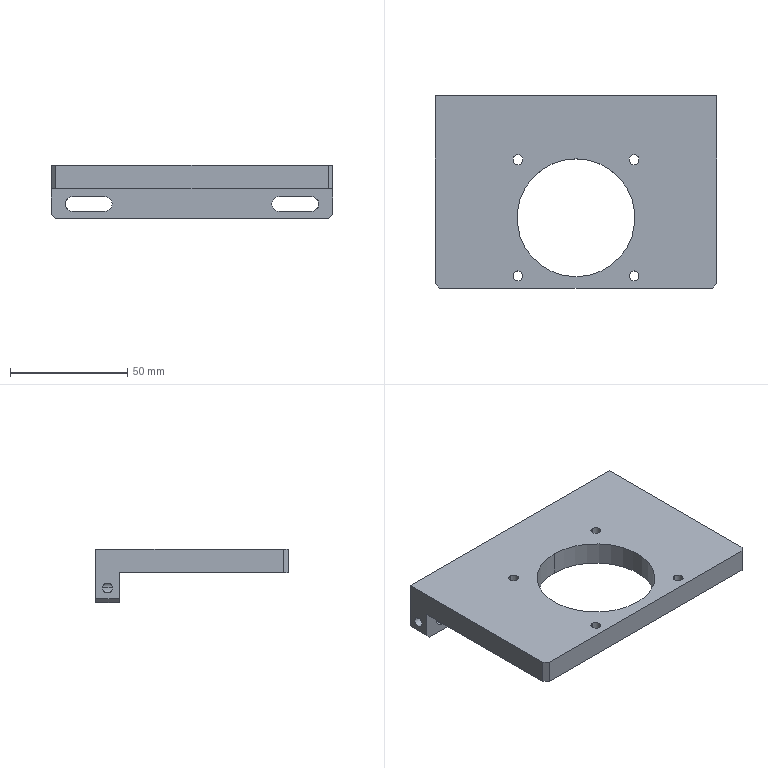NC program | NX | posted with a generic post | part box 120 x 82 x 22.8 mm
Lines 23 to 861 of 3479:
(ZLEVEL_PROFILE , TOOL : D10)
N44 T15 M6
N46 G54
N48 G17 G0 G90 X-47.537 Y46.1 B0. C0. S9500 M3
N50 G43 Z30. H15
N52 Z1.5
N54 G94 G1 X0. Z-0.991 F1000.
N56 X60. F3000.
N58 G2 X65.1 Y41. R5.1
N60 G1 Y-39.
N62 G2 X63.606 Y-42.606 R5.1
N64 G1 X61.606 Y-44.606
N66 G2 X58. Y-46.1 R5.1
N68 G1 X-58.
N70 G2 X-61.606 Y-44.606 R5.1
N72 G1 X-63.606 Y-42.606
N74 G2 X-65.1 Y-39. R5.1
N76 G1 Y41.
N78 G2 X-60. Y46.1 R5.1
N80 G1 X0.
N82 X60. Z-1.128
N84 X60.5 Y46.075 Z-1.13
N86 X60.995 Y46.002 Z-1.131
N88 X61.48 Y45.88 Z-1.132
N90 X61.952 Y45.712 Z-1.133
N92 X62.404 Y45.498 Z-1.134
N94 X62.833 Y45.24 Z-1.135
N96 X63.235 Y44.942 Z-1.136
N98 X63.606 Y44.606 Z-1.138
N100 X63.942 Y44.235 Z-1.139
N102 X64.24 Y43.833 Z-1.14
N104 X64.498 Y43.404 Z-1.141
N106 X64.712 Y42.952 Z-1.142
N108 X64.88 Y42.48 Z-1.143
N110 X65.002 Y41.995 Z-1.144
N112 X65.075 Y41.5 Z-1.146
N114 X65.1 Y41. Z-1.147
N116 Y-39. Z-1.33
N118 X65.075 Y-39.5 Z-1.331
N120 X65.002 Y-39.995 Z-1.332
N122 X64.88 Y-40.48 Z-1.333
N124 X64.712 Y-40.952 Z-1.334
N126 X64.498 Y-41.404 Z-1.335
N128 X64.24 Y-41.833 Z-1.336
N130 X63.942 Y-42.235 Z-1.338
N132 X63.606 Y-42.606 Z-1.339
N134 X61.606 Y-44.606 Z-1.345
N136 X61.235 Y-44.942 Z-1.346
N138 X60.833 Y-45.24 Z-1.348
N140 X60.404 Y-45.498 Z-1.349
N142 X59.952 Y-45.712 Z-1.35
N144 X59.48 Y-45.88 Z-1.351
N146 X58.995 Y-46.002 Z-1.352
N148 X58.5 Y-46.075 Z-1.353
N150 X58. Y-46.1 Z-1.354
N152 X-58. Z-1.62
N154 X-58.5 Y-46.075 Z-1.621
N156 X-58.995 Y-46.002 Z-1.622
N158 X-59.48 Y-45.88 Z-1.623
N160 X-59.952 Y-45.712 Z-1.624
N162 X-60.404 Y-45.498 Z-1.625
N164 X-60.833 Y-45.24 Z-1.626
N166 X-61.235 Y-44.942 Z-1.628
N168 X-61.606 Y-44.606 Z-1.629
N170 X-63.606 Y-42.606 Z-1.635
N172 X-63.942 Y-42.235 Z-1.636
N174 X-64.24 Y-41.833 Z-1.637
N176 X-64.498 Y-41.404 Z-1.639
N178 X-64.712 Y-40.952 Z-1.64
N180 X-64.88 Y-40.48 Z-1.641
N182 X-65.002 Y-39.995 Z-1.642
N184 X-65.075 Y-39.5 Z-1.643
N186 X-65.1 Y-39. Z-1.644
N188 Y41. Z-1.827
N190 X-65.075 Y41.5 Z-1.828
N192 X-65.002 Y41.995 Z-1.829
N194 X-64.88 Y42.48 Z-1.831
N196 X-64.712 Y42.952 Z-1.832
N198 X-64.498 Y43.404 Z-1.833
N200 X-64.24 Y43.833 Z-1.834
N202 X-63.942 Y44.235 Z-1.835
N204 X-63.606 Y44.606 Z-1.836
N206 X-63.235 Y44.942 Z-1.837
N208 X-62.833 Y45.24 Z-1.839
N210 X-62.404 Y45.498 Z-1.84
N212 X-61.952 Y45.712 Z-1.841
N214 X-61.48 Y45.88 Z-1.842
N216 X-60.995 Y46.002 Z-1.843
N218 X-60.5 Y46.075 Z-1.844
N220 X-60. Y46.1 Z-1.845
N222 X0. Z-1.983
N224 X60. Z-2.12
N226 X60.5 Y46.075 Z-2.121
N228 X60.995 Y46.002 Z-2.122
N230 X61.48 Y45.88 Z-2.123
N232 X61.952 Y45.712 Z-2.124
N234 X62.404 Y45.498 Z-2.125
N236 X62.833 Y45.24 Z-2.127
N238 X63.235 Y44.942 Z-2.128
N240 X63.606 Y44.606 Z-2.129
N242 X63.942 Y44.235 Z-2.13
N244 X64.24 Y43.833 Z-2.131
N246 X64.498 Y43.404 Z-2.132
N248 X64.712 Y42.952 Z-2.133
N250 X64.88 Y42.48 Z-2.135
N252 X65.002 Y41.995 Z-2.136
N254 X65.075 Y41.5 Z-2.137
N256 X65.1 Y41. Z-2.138
N258 Y-39. Z-2.321
N260 X65.075 Y-39.5 Z-2.322
N262 X65.002 Y-39.995 Z-2.323
N264 X64.88 Y-40.48 Z-2.324
N266 X64.712 Y-40.952 Z-2.325
N268 X64.498 Y-41.404 Z-2.327
N270 X64.24 Y-41.833 Z-2.328
N272 X63.942 Y-42.235 Z-2.329
N274 X63.606 Y-42.606 Z-2.33
N276 X61.606 Y-44.606 Z-2.337
N278 X61.235 Y-44.942 Z-2.338
N280 X60.833 Y-45.24 Z-2.339
N282 X60.404 Y-45.498 Z-2.34
N284 X59.952 Y-45.712 Z-2.341
N286 X59.48 Y-45.88 Z-2.342
N288 X58.995 Y-46.002 Z-2.343
N290 X58.5 Y-46.075 Z-2.345
N292 X58. Y-46.1 Z-2.346
N294 X-58. Z-2.611
N296 X-58.5 Y-46.075 Z-2.612
N298 X-58.995 Y-46.002 Z-2.613
N300 X-59.48 Y-45.88 Z-2.614
N302 X-59.952 Y-45.712 Z-2.615
N304 X-60.404 Y-45.498 Z-2.617
N306 X-60.833 Y-45.24 Z-2.618
N308 X-61.235 Y-44.942 Z-2.619
N310 X-61.606 Y-44.606 Z-2.62
N312 X-63.606 Y-42.606 Z-2.626
N314 X-63.942 Y-42.235 Z-2.628
N316 X-64.24 Y-41.833 Z-2.629
N318 X-64.498 Y-41.404 Z-2.63
N320 X-64.712 Y-40.952 Z-2.631
N322 X-64.88 Y-40.48 Z-2.632
N324 X-65.002 Y-39.995 Z-2.633
N326 X-65.075 Y-39.5 Z-2.634
N328 X-65.1 Y-39. Z-2.636
N330 Y41. Z-2.818
N332 X-65.075 Y41.5 Z-2.82
N334 X-65.002 Y41.995 Z-2.821
N336 X-64.88 Y42.48 Z-2.822
N338 X-64.712 Y42.952 Z-2.823
N340 X-64.498 Y43.404 Z-2.824
N342 X-64.24 Y43.833 Z-2.825
N344 X-63.942 Y44.235 Z-2.826
N346 X-63.606 Y44.606 Z-2.828
N348 X-63.235 Y44.942 Z-2.829
N350 X-62.833 Y45.24 Z-2.83
N352 X-62.404 Y45.498 Z-2.831
N354 X-61.952 Y45.712 Z-2.832
N356 X-61.48 Y45.88 Z-2.833
N358 X-60.995 Y46.002 Z-2.834
N360 X-60.5 Y46.075 Z-2.836
N362 X-60. Y46.1 Z-2.837
N364 X0. Z-2.974
N366 X60. Z-3.111
N368 X60.5 Y46.075 Z-3.112
N370 X60.995 Y46.002 Z-3.113
N372 X61.48 Y45.88 Z-3.114
N374 X61.952 Y45.712 Z-3.116
N376 X62.404 Y45.498 Z-3.117
N378 X62.833 Y45.24 Z-3.118
N380 X63.235 Y44.942 Z-3.119
N382 X63.606 Y44.606 Z-3.12
N384 X63.942 Y44.235 Z-3.121
N386 X64.24 Y43.833 Z-3.122
N388 X64.498 Y43.404 Z-3.124
N390 X64.712 Y42.952 Z-3.125
N392 X64.88 Y42.48 Z-3.126
N394 X65.002 Y41.995 Z-3.127
N396 X65.075 Y41.5 Z-3.128
N398 X65.1 Y41. Z-3.129
N400 Y-39. Z-3.312
N402 X65.075 Y-39.5 Z-3.313
N404 X65.002 Y-39.995 Z-3.315
N406 X64.88 Y-40.48 Z-3.316
N408 X64.712 Y-40.952 Z-3.317
N410 X64.498 Y-41.404 Z-3.318
N412 X64.24 Y-41.833 Z-3.319
N414 X63.942 Y-42.235 Z-3.32
N416 X63.606 Y-42.606 Z-3.321
N418 X61.606 Y-44.606 Z-3.328
N420 X61.235 Y-44.942 Z-3.329
N422 X60.833 Y-45.24 Z-3.33
N424 X60.404 Y-45.498 Z-3.331
N426 X59.952 Y-45.712 Z-3.332
N428 X59.48 Y-45.88 Z-3.334
N430 X58.995 Y-46.002 Z-3.335
N432 X58.5 Y-46.075 Z-3.336
N434 X58. Y-46.1 Z-3.337
N436 X-58. Z-3.602
N438 X-58.5 Y-46.075 Z-3.603
N440 X-58.995 Y-46.002 Z-3.604
N442 X-59.48 Y-45.88 Z-3.606
N444 X-59.952 Y-45.712 Z-3.607
N446 X-60.404 Y-45.498 Z-3.608
N448 X-60.833 Y-45.24 Z-3.609
N450 X-61.235 Y-44.942 Z-3.61
N452 X-61.606 Y-44.606 Z-3.611
N454 X-63.606 Y-42.606 Z-3.618
N456 X-63.942 Y-42.235 Z-3.619
N458 X-64.24 Y-41.833 Z-3.62
N460 X-64.498 Y-41.404 Z-3.621
N462 X-64.712 Y-40.952 Z-3.622
N464 X-64.88 Y-40.48 Z-3.623
N466 X-65.002 Y-39.995 Z-3.625
N468 X-65.075 Y-39.5 Z-3.626
N470 X-65.1 Y-39. Z-3.627
N472 Y41. Z-3.81
N474 X-65.075 Y41.5 Z-3.811
N476 X-65.002 Y41.995 Z-3.812
N478 X-64.88 Y42.48 Z-3.813
N480 X-64.712 Y42.952 Z-3.814
N482 X-64.498 Y43.404 Z-3.815
N484 X-64.24 Y43.833 Z-3.817
N486 X-63.942 Y44.235 Z-3.818
N488 X-63.606 Y44.606 Z-3.819
N490 X-63.235 Y44.942 Z-3.82
N492 X-62.833 Y45.24 Z-3.821
N494 X-62.404 Y45.498 Z-3.822
N496 X-61.952 Y45.712 Z-3.823
N498 X-61.48 Y45.88 Z-3.825
N500 X-60.995 Y46.002 Z-3.826
N502 X-60.5 Y46.075 Z-3.827
N504 X-60. Y46.1 Z-3.828
N506 X0. Z-3.965
N508 X60. Z-4.102
N510 X60.5 Y46.075 Z-4.104
N512 X60.995 Y46.002 Z-4.105
N514 X61.48 Y45.88 Z-4.106
N516 X61.952 Y45.712 Z-4.107
N518 X62.404 Y45.498 Z-4.108
N520 X62.833 Y45.24 Z-4.109
N522 X63.235 Y44.942 Z-4.11
N524 X63.606 Y44.606 Z-4.112
N526 X63.942 Y44.235 Z-4.113
N528 X64.24 Y43.833 Z-4.114
N530 X64.498 Y43.404 Z-4.115
N532 X64.712 Y42.952 Z-4.116
N534 X64.88 Y42.48 Z-4.117
N536 X65.002 Y41.995 Z-4.118
N538 X65.075 Y41.5 Z-4.12
N540 X65.1 Y41. Z-4.121
N542 Y-39. Z-4.304
N544 X65.075 Y-39.5 Z-4.305
N546 X65.002 Y-39.995 Z-4.306
N548 X64.88 Y-40.48 Z-4.307
N550 X64.712 Y-40.952 Z-4.308
N552 X64.498 Y-41.404 Z-4.309
N554 X64.24 Y-41.833 Z-4.31
N556 X63.942 Y-42.235 Z-4.312
N558 X63.606 Y-42.606 Z-4.313
N560 X61.606 Y-44.606 Z-4.319
N562 X61.235 Y-44.942 Z-4.32
N564 X60.833 Y-45.24 Z-4.321
N566 X60.404 Y-45.498 Z-4.323
N568 X59.952 Y-45.712 Z-4.324
N570 X59.48 Y-45.88 Z-4.325
N572 X58.995 Y-46.002 Z-4.326
N574 X58.5 Y-46.075 Z-4.327
N576 X58. Y-46.1 Z-4.328
N578 X-58. Z-4.593
N580 X-58.5 Y-46.075 Z-4.595
N582 X-58.995 Y-46.002 Z-4.596
N584 X-59.48 Y-45.88 Z-4.597
N586 X-59.952 Y-45.712 Z-4.598
N588 X-60.404 Y-45.498 Z-4.599
N590 X-60.833 Y-45.24 Z-4.6
N592 X-61.235 Y-44.942 Z-4.601
N594 X-61.606 Y-44.606 Z-4.603
N596 X-63.606 Y-42.606 Z-4.609
N598 X-63.942 Y-42.235 Z-4.61
N600 X-64.24 Y-41.833 Z-4.611
N602 X-64.498 Y-41.404 Z-4.612
N604 X-64.712 Y-40.952 Z-4.614
N606 X-64.88 Y-40.48 Z-4.615
N608 X-65.002 Y-39.995 Z-4.616
N610 X-65.075 Y-39.5 Z-4.617
N612 X-65.1 Y-39. Z-4.618
N614 Y41. Z-4.801
N616 X-65.075 Y41.5 Z-4.802
N618 X-65.002 Y41.995 Z-4.803
N620 X-64.88 Y42.48 Z-4.805
N622 X-64.712 Y42.952 Z-4.806
N624 X-64.498 Y43.404 Z-4.807
N626 X-64.24 Y43.833 Z-4.808
N628 X-63.942 Y44.235 Z-4.809
N630 X-63.606 Y44.606 Z-4.81
N632 X-63.235 Y44.942 Z-4.811
N634 X-62.833 Y45.24 Z-4.813
N636 X-62.404 Y45.498 Z-4.814
N638 X-61.952 Y45.712 Z-4.815
N640 X-61.48 Y45.88 Z-4.816
N642 X-60.995 Y46.002 Z-4.817
N644 X-60.5 Y46.075 Z-4.818
N646 X-60. Y46.1 Z-4.819
N648 X0. Z-4.957
N650 X60. Z-5.094
N652 X60.5 Y46.075 Z-5.095
N654 X60.995 Y46.002 Z-5.096
N656 X61.48 Y45.88 Z-5.097
N658 X61.952 Y45.712 Z-5.098
N660 X62.404 Y45.498 Z-5.099
N662 X62.833 Y45.24 Z-5.101
N664 X63.235 Y44.942 Z-5.102
N666 X63.606 Y44.606 Z-5.103
N668 X63.942 Y44.235 Z-5.104
N670 X64.24 Y43.833 Z-5.105
N672 X64.498 Y43.404 Z-5.106
N674 X64.712 Y42.952 Z-5.107
N676 X64.88 Y42.48 Z-5.109
N678 X65.002 Y41.995 Z-5.11
N680 X65.075 Y41.5 Z-5.111
N682 X65.1 Y41. Z-5.112
N684 Y-39. Z-5.295
N686 X65.075 Y-39.5 Z-5.296
N688 X65.002 Y-39.995 Z-5.297
N690 X64.88 Y-40.48 Z-5.298
N692 X64.712 Y-40.952 Z-5.299
N694 X64.498 Y-41.404 Z-5.301
N696 X64.24 Y-41.833 Z-5.302
N698 X63.942 Y-42.235 Z-5.303
N700 X63.606 Y-42.606 Z-5.304
N702 X61.606 Y-44.606 Z-5.31
N704 X61.235 Y-44.942 Z-5.312
N706 X60.833 Y-45.24 Z-5.313
N708 X60.404 Y-45.498 Z-5.314
N710 X59.952 Y-45.712 Z-5.315
N712 X59.48 Y-45.88 Z-5.316
N714 X58.995 Y-46.002 Z-5.317
N716 X58.5 Y-46.075 Z-5.318
N718 X58. Y-46.1 Z-5.32
N720 X-58. Z-5.585
N722 X-58.5 Y-46.075 Z-5.586
N724 X-58.995 Y-46.002 Z-5.587
N726 X-59.48 Y-45.88 Z-5.588
N728 X-59.952 Y-45.712 Z-5.589
N730 X-60.404 Y-45.498 Z-5.59
N732 X-60.833 Y-45.24 Z-5.592
N734 X-61.235 Y-44.942 Z-5.593
N736 X-61.606 Y-44.606 Z-5.594
N738 X-63.606 Y-42.606 Z-5.6
N740 X-63.942 Y-42.235 Z-5.602
N742 X-64.24 Y-41.833 Z-5.603
N744 X-64.498 Y-41.404 Z-5.604
N746 X-64.712 Y-40.952 Z-5.605
N748 X-64.88 Y-40.48 Z-5.606
N750 X-65.002 Y-39.995 Z-5.607
N752 X-65.075 Y-39.5 Z-5.608
N754 X-65.1 Y-39. Z-5.61
N756 Y41. Z-5.792
N758 X-65.075 Y41.5 Z-5.794
N760 X-65.002 Y41.995 Z-5.795
N762 X-64.88 Y42.48 Z-5.796
N764 X-64.712 Y42.952 Z-5.797
N766 X-64.498 Y43.404 Z-5.798
N768 X-64.24 Y43.833 Z-5.799
N770 X-63.942 Y44.235 Z-5.8
N772 X-63.606 Y44.606 Z-5.802
N774 X-63.235 Y44.942 Z-5.803
N776 X-62.833 Y45.24 Z-5.804
N778 X-62.404 Y45.498 Z-5.805
N780 X-61.952 Y45.712 Z-5.806
N782 X-61.48 Y45.88 Z-5.807
N784 X-60.995 Y46.002 Z-5.808
N786 X-60.5 Y46.075 Z-5.81
N788 X-60. Y46.1 Z-5.811
N790 X0. Z-5.948
N792 X60. Z-6.085
N794 X60.5 Y46.075 Z-6.086
N796 X60.995 Y46.002 Z-6.087
N798 X61.48 Y45.88 Z-6.088
N800 X61.952 Y45.712 Z-6.09
N802 X62.404 Y45.498 Z-6.091
N804 X62.833 Y45.24 Z-6.092
N806 X63.235 Y44.942 Z-6.093
N808 X63.606 Y44.606 Z-6.094
N810 X63.942 Y44.235 Z-6.095
N812 X64.24 Y43.833 Z-6.096
N814 X64.498 Y43.404 Z-6.098
N816 X64.712 Y42.952 Z-6.099
N818 X64.88 Y42.48 Z-6.1
N820 X65.002 Y41.995 Z-6.101
N822 X65.075 Y41.5 Z-6.102
N824 X65.1 Y41. Z-6.103
N826 Y-39. Z-6.286
N828 X65.075 Y-39.5 Z-6.287
N830 X65.002 Y-39.995 Z-6.288
N832 X64.88 Y-40.48 Z-6.29
N834 X64.712 Y-40.952 Z-6.291
N836 X64.498 Y-41.404 Z-6.292
N838 X64.24 Y-41.833 Z-6.293
N840 X63.942 Y-42.235 Z-6.294
N842 X63.606 Y-42.606 Z-6.295
N844 X61.606 Y-44.606 Z-6.302
N846 X61.235 Y-44.942 Z-6.303
N848 X60.833 Y-45.24 Z-6.304
N850 X60.404 Y-45.498 Z-6.305
N852 X59.952 Y-45.712 Z-6.306
N854 X59.48 Y-45.88 Z-6.307
N856 X58.995 Y-46.002 Z-6.309
N858 X58.5 Y-46.075 Z-6.31
N860 X58. Y-46.1 Z-6.311
N862 X-58. Z-6.576
N864 X-58.5 Y-46.075 Z-6.577
N866 X-58.995 Y-46.002 Z-6.578
N868 X-59.48 Y-45.88 Z-6.579
N870 X-59.952 Y-45.712 Z-6.581
N872 X-60.404 Y-45.498 Z-6.582
N874 X-60.833 Y-45.24 Z-6.583
N876 X-61.235 Y-44.942 Z-6.584
N878 X-61.606 Y-44.606 Z-6.585
N880 X-63.606 Y-42.606 Z-6.592
N882 X-63.942 Y-42.235 Z-6.593
N884 X-64.24 Y-41.833 Z-6.594
N886 X-64.498 Y-41.404 Z-6.595
N888 X-64.712 Y-40.952 Z-6.596
N890 X-64.88 Y-40.48 Z-6.597
N892 X-65.002 Y-39.995 Z-6.599
N894 X-65.075 Y-39.5 Z-6.6
N896 X-65.1 Y-39. Z-6.601
N898 Y41. Z-6.784
N900 X-65.075 Y41.5 Z-6.785
N902 X-65.002 Y41.995 Z-6.786
N904 X-64.88 Y42.48 Z-6.787
N906 X-64.712 Y42.952 Z-6.788
N908 X-64.498 Y43.404 Z-6.789
N910 X-64.24 Y43.833 Z-6.791
N912 X-63.942 Y44.235 Z-6.792
N914 X-63.606 Y44.606 Z-6.793
N916 X-63.235 Y44.942 Z-6.794
N918 X-62.833 Y45.24 Z-6.795
N920 X-62.404 Y45.498 Z-6.796
N922 X-61.952 Y45.712 Z-6.797
N924 X-61.48 Y45.88 Z-6.799
N926 X-60.995 Y46.002 Z-6.8
N928 X-60.5 Y46.075 Z-6.801
N930 X-60. Y46.1 Z-6.802
N932 X0. Z-6.939
N934 X60. Z-7.076
N936 X60.5 Y46.075 Z-7.077
N938 X60.995 Y46.002 Z-7.079
N940 X61.48 Y45.88 Z-7.08
N942 X61.952 Y45.712 Z-7.081
N944 X62.404 Y45.498 Z-7.082
N946 X62.833 Y45.24 Z-7.083
N948 X63.235 Y44.942 Z-7.084
N950 X63.606 Y44.606 Z-7.085
N952 X63.942 Y44.235 Z-7.087
N954 X64.24 Y43.833 Z-7.088
N956 X64.498 Y43.404 Z-7.089
N958 X64.712 Y42.952 Z-7.09
N960 X64.88 Y42.48 Z-7.091
N962 X65.002 Y41.995 Z-7.092
N964 X65.075 Y41.5 Z-7.093
N966 X65.1 Y41. Z-7.095
N968 Y-39. Z-7.277
N970 X65.075 Y-39.5 Z-7.279
N972 X65.002 Y-39.995 Z-7.28
N974 X64.88 Y-40.48 Z-7.281
N976 X64.712 Y-40.952 Z-7.282
N978 X64.498 Y-41.404 Z-7.283
N980 X64.24 Y-41.833 Z-7.284
N982 X63.942 Y-42.235 Z-7.285
N984 X63.606 Y-42.606 Z-7.287
N986 X61.606 Y-44.606 Z-7.293
N988 X61.235 Y-44.942 Z-7.294
N990 X60.833 Y-45.24 Z-7.295
N992 X60.404 Y-45.498 Z-7.296
N994 X59.952 Y-45.712 Z-7.298
N996 X59.48 Y-45.88 Z-7.299
N998 X58.995 Y-46.002 Z-7.3
N1000 X58.5 Y-46.075 Z-7.301
N1002 X58. Y-46.1 Z-7.302
N1004 X-58. Z-7.567
N1006 X-58.5 Y-46.075 Z-7.569
N1008 X-58.995 Y-46.002 Z-7.57
N1010 X-59.48 Y-45.88 Z-7.571
N1012 X-59.952 Y-45.712 Z-7.572
N1014 X-60.404 Y-45.498 Z-7.573
N1016 X-60.833 Y-45.24 Z-7.574
N1018 X-61.235 Y-44.942 Z-7.575
N1020 X-61.606 Y-44.606 Z-7.577
N1022 X-63.606 Y-42.606 Z-7.583
N1024 X-63.942 Y-42.235 Z-7.584
N1026 X-64.24 Y-41.833 Z-7.585
N1028 X-64.498 Y-41.404 Z-7.586
N1030 X-64.712 Y-40.952 Z-7.588
N1032 X-64.88 Y-40.48 Z-7.589
N1034 X-65.002 Y-39.995 Z-7.59
N1036 X-65.075 Y-39.5 Z-7.591
N1038 X-65.1 Y-39. Z-7.592
N1040 Y41. Z-7.775
N1042 X-65.075 Y41.5 Z-7.776
N1044 X-65.002 Y41.995 Z-7.777
N1046 X-64.88 Y42.48 Z-7.778
N1048 X-64.712 Y42.952 Z-7.78
N1050 X-64.498 Y43.404 Z-7.781
N1052 X-64.24 Y43.833 Z-7.782
N1054 X-63.942 Y44.235 Z-7.783
N1056 X-63.606 Y44.606 Z-7.784
N1058 X-63.235 Y44.942 Z-7.785
N1060 X-62.833 Y45.24 Z-7.786
N1062 X-62.404 Y45.498 Z-7.788
N1064 X-61.952 Y45.712 Z-7.789
N1066 X-61.48 Y45.88 Z-7.79
N1068 X-60.995 Y46.002 Z-7.791
N1070 X-60.5 Y46.075 Z-7.792
N1072 X-60. Y46.1 Z-7.793
N1074 X0. Z-7.93
N1076 X60. Z-8.068
N1078 X60.5 Y46.075 Z-8.069
N1080 X60.995 Y46.002 Z-8.07
N1082 X61.48 Y45.88 Z-8.071
N1084 X61.952 Y45.712 Z-8.072
N1086 X62.404 Y45.498 Z-8.073
N1088 X62.833 Y45.24 Z-8.074
N1090 X63.235 Y44.942 Z-8.076
N1092 X63.606 Y44.606 Z-8.077
N1094 X63.942 Y44.235 Z-8.078
N1096 X64.24 Y43.833 Z-8.079
N1098 X64.498 Y43.404 Z-8.08
N1100 X64.712 Y42.952 Z-8.081
N1102 X64.88 Y42.48 Z-8.082
N1104 X65.002 Y41.995 Z-8.084
N1106 X65.075 Y41.5 Z-8.085
N1108 X65.1 Y41. Z-8.086
N1110 Y-39. Z-8.269
N1112 X65.075 Y-39.5 Z-8.27
N1114 X65.002 Y-39.995 Z-8.271
N1116 X64.88 Y-40.48 Z-8.272
N1118 X64.712 Y-40.952 Z-8.273
N1120 X64.498 Y-41.404 Z-8.274
N1122 X64.24 Y-41.833 Z-8.276
N1124 X63.942 Y-42.235 Z-8.277
N1126 X63.606 Y-42.606 Z-8.278
N1128 X61.606 Y-44.606 Z-8.284
N1130 X61.235 Y-44.942 Z-8.286
N1132 X60.833 Y-45.24 Z-8.287
N1134 X60.404 Y-45.498 Z-8.288
N1136 X59.952 Y-45.712 Z-8.289
N1138 X59.48 Y-45.88 Z-8.29
N1140 X58.995 Y-46.002 Z-8.291
N1142 X58.5 Y-46.075 Z-8.292
N1144 X58. Y-46.1 Z-8.294
N1146 X-58. Z-8.559
N1148 X-58.5 Y-46.075 Z-8.56
N1150 X-58.995 Y-46.002 Z-8.561
N1152 X-59.48 Y-45.88 Z-8.562
N1154 X-59.952 Y-45.712 Z-8.563
N1156 X-60.404 Y-45.498 Z-8.564
N1158 X-60.833 Y-45.24 Z-8.566
N1160 X-61.235 Y-44.942 Z-8.567
N1162 X-61.606 Y-44.606 Z-8.568
N1164 X-63.606 Y-42.606 Z-8.574
N1166 X-63.942 Y-42.235 Z-8.575
N1168 X-64.24 Y-41.833 Z-8.577
N1170 X-64.498 Y-41.404 Z-8.578
N1172 X-64.712 Y-40.952 Z-8.579
N1174 X-64.88 Y-40.48 Z-8.58
N1176 X-65.002 Y-39.995 Z-8.581
N1178 X-65.075 Y-39.5 Z-8.582
N1180 X-65.1 Y-39. Z-8.583
N1182 Y41. Z-8.766
N1184 X-65.075 Y41.5 Z-8.767
N1186 X-65.002 Y41.995 Z-8.769
N1188 X-64.88 Y42.48 Z-8.77
N1190 X-64.712 Y42.952 Z-8.771
N1192 X-64.498 Y43.404 Z-8.772
N1194 X-64.24 Y43.833 Z-8.773
N1196 X-63.942 Y44.235 Z-8.774
N1198 X-63.606 Y44.606 Z-8.775
N1200 X-63.235 Y44.942 Z-8.777
N1202 X-62.833 Y45.24 Z-8.778
N1204 X-62.404 Y45.498 Z-8.779
N1206 X-61.952 Y45.712 Z-8.78
N1208 X-61.48 Y45.88 Z-8.781
N1210 X-60.995 Y46.002 Z-8.782
N1212 X-60.5 Y46.075 Z-8.783
N1214 X-60. Y46.1 Z-8.785
N1216 X0. Z-8.922
N1218 X60. Z-9.059
N1220 X60.5 Y46.075 Z-9.06
N1222 X60.995 Y46.002 Z-9.061
N1224 X61.48 Y45.88 Z-9.062
N1226 X61.952 Y45.712 Z-9.063
N1228 X62.404 Y45.498 Z-9.065
N1230 X62.833 Y45.24 Z-9.066
N1232 X63.235 Y44.942 Z-9.067
N1234 X63.606 Y44.606 Z-9.068
N1236 X63.942 Y44.235 Z-9.069
N1238 X64.24 Y43.833 Z-9.07
N1240 X64.498 Y43.404 Z-9.071
N1242 X64.712 Y42.952 Z-9.073
N1244 X64.88 Y42.48 Z-9.074
N1246 X65.002 Y41.995 Z-9.075
N1248 X65.075 Y41.5 Z-9.076
N1250 X65.1 Y41. Z-9.077
N1252 Y-39. Z-9.26
N1254 X65.075 Y-39.5 Z-9.261
N1256 X65.002 Y-39.995 Z-9.262
N1258 X64.88 Y-40.48 Z-9.263
N1260 X64.712 Y-40.952 Z-9.265
N1262 X64.498 Y-41.404 Z-9.266
N1264 X64.24 Y-41.833 Z-9.267
N1266 X63.942 Y-42.235 Z-9.268
N1268 X63.606 Y-42.606 Z-9.269
N1270 X61.606 Y-44.606 Z-9.276
N1272 X61.235 Y-44.942 Z-9.277
N1274 X60.833 Y-45.24 Z-9.278
N1276 X60.404 Y-45.498 Z-9.279
N1278 X59.952 Y-45.712 Z-9.28
N1280 X59.48 Y-45.88 Z-9.281
N1282 X58.995 Y-46.002 Z-9.283
N1284 X58.5 Y-46.075 Z-9.284
N1286 X58. Y-46.1 Z-9.285
N1288 X-58. Z-9.55
N1290 X-58.5 Y-46.075 Z-9.551
N1292 X-58.995 Y-46.002 Z-9.552
N1294 X-59.48 Y-45.88 Z-9.553
N1296 X-59.952 Y-45.712 Z-9.555
N1298 X-60.404 Y-45.498 Z-9.556
N1300 X-60.833 Y-45.24 Z-9.557
N1302 X-61.235 Y-44.942 Z-9.558
N1304 X-61.606 Y-44.606 Z-9.559
N1306 X-63.606 Y-42.606 Z-9.566
N1308 X-63.942 Y-42.235 Z-9.567
N1310 X-64.24 Y-41.833 Z-9.568
N1312 X-64.498 Y-41.404 Z-9.569
N1314 X-64.712 Y-40.952 Z-9.57
N1316 X-64.88 Y-40.48 Z-9.571
N1318 X-65.002 Y-39.995 Z-9.572
N1320 X-65.075 Y-39.5 Z-9.574
N1322 X-65.1 Y-39. Z-9.575
N1324 Y41. Z-9.758
N1326 X-65.075 Y41.5 Z-9.759
N1328 X-65.002 Y41.995 Z-9.76
N1330 X-64.88 Y42.48 Z-9.761
N1332 X-64.712 Y42.952 Z-9.762
N1334 X-64.498 Y43.404 Z-9.763
N1336 X-64.24 Y43.833 Z-9.764
N1338 X-63.942 Y44.235 Z-9.766
N1340 X-63.606 Y44.606 Z-9.767
N1342 X-63.235 Y44.942 Z-9.768
N1344 X-62.833 Y45.24 Z-9.769
N1346 X-62.404 Y45.498 Z-9.77
N1348 X-61.952 Y45.712 Z-9.771
N1350 X-61.48 Y45.88 Z-9.772
N1352 X-60.995 Y46.002 Z-9.774
N1354 X-60.5 Y46.075 Z-9.775
N1356 X-60. Y46.1 Z-9.776
N1358 X0. Z-9.913
N1360 X60. Z-10.05
N1362 X60.5 Y46.075 Z-10.051
N1364 X60.995 Y46.002 Z-10.052
N1366 X61.48 Y45.88 Z-10.054
N1368 X61.952 Y45.712 Z-10.055
N1370 X62.404 Y45.498 Z-10.056
N1372 X62.833 Y45.24 Z-10.057
N1374 X63.235 Y44.942 Z-10.058
N1376 X63.606 Y44.606 Z-10.059
N1378 X63.942 Y44.235 Z-10.06
N1380 X64.24 Y43.833 Z-10.062
N1382 X64.498 Y43.404 Z-10.063
N1384 X64.712 Y42.952 Z-10.064
N1386 X64.88 Y42.48 Z-10.065
N1388 X65.002 Y41.995 Z-10.066
N1390 X65.075 Y41.5 Z-10.067
N1392 X65.1 Y41. Z-10.068
N1394 Y-39. Z-10.251
N1396 X65.075 Y-39.5 Z-10.253
N1398 X65.002 Y-39.995 Z-10.254
N1400 X64.88 Y-40.48 Z-10.255
N1402 X64.712 Y-40.952 Z-10.256
N1404 X64.498 Y-41.404 Z-10.257
N1406 X64.24 Y-41.833 Z-10.258
N1408 X63.942 Y-42.235 Z-10.259
N1410 X63.606 Y-42.606 Z-10.261
N1412 X61.606 Y-44.606 Z-10.267
N1414 X61.235 Y-44.942 Z-10.268
N1416 X60.833 Y-45.24 Z-10.269
N1418 X60.404 Y-45.498 Z-10.27
N1420 X59.952 Y-45.712 Z-10.272
N1422 X59.48 Y-45.88 Z-10.273
N1424 X58.995 Y-46.002 Z-10.274
N1426 X58.5 Y-46.075 Z-10.275
N1428 X58. Y-46.1 Z-10.276
N1430 X-58. Z-10.541
N1432 X-58.5 Y-46.075 Z-10.542
N1434 X-58.995 Y-46.002 Z-10.544
N1436 X-59.48 Y-45.88 Z-10.545
N1438 X-59.952 Y-45.712 Z-10.546
N1440 X-60.404 Y-45.498 Z-10.547
N1442 X-60.833 Y-45.24 Z-10.548
N1444 X-61.235 Y-44.942 Z-10.549
N1446 X-61.606 Y-44.606 Z-10.55
N1448 X-63.606 Y-42.606 Z-10.557
N1450 X-63.942 Y-42.235 Z-10.558
N1452 X-64.24 Y-41.833 Z-10.559
N1454 X-64.498 Y-41.404 Z-10.56
N1456 X-64.712 Y-40.952 Z-10.561
N1458 X-64.88 Y-40.48 Z-10.563
N1460 X-65.002 Y-39.995 Z-10.564
N1462 X-65.075 Y-39.5 Z-10.565
N1464 X-65.1 Y-39. Z-10.566
N1466 Y41. Z-10.749
N1468 X-65.075 Y41.5 Z-10.75
N1470 X-65.002 Y41.995 Z-10.751
N1472 X-64.88 Y42.48 Z-10.752
N1474 X-64.712 Y42.952 Z-10.753
N1476 X-64.498 Y43.404 Z-10.755
N1478 X-64.24 Y43.833 Z-10.756
N1480 X-63.942 Y44.235 Z-10.757
N1482 X-63.606 Y44.606 Z-10.758
N1484 X-63.235 Y44.942 Z-10.759
N1486 X-62.833 Y45.24 Z-10.76
N1488 X-62.404 Y45.498 Z-10.761
N1490 X-61.952 Y45.712 Z-10.763
N1492 X-61.48 Y45.88 Z-10.764
N1494 X-60.995 Y46.002 Z-10.765
N1496 X-60.5 Y46.075 Z-10.766
N1498 X-60. Y46.1 Z-10.767
N1500 X0. Z-10.904
N1502 X60. Z-11.042
N1504 X60.5 Y46.075 Z-11.043
N1506 X60.995 Y46.002 Z-11.044
N1508 X61.48 Y45.88 Z-11.045
N1510 X61.952 Y45.712 Z-11.046
N1512 X62.404 Y45.498 Z-11.047
N1514 X62.833 Y45.24 Z-11.048
N1516 X63.235 Y44.942 Z-11.05
N1518 X63.606 Y44.606 Z-11.051
N1520 X63.942 Y44.235 Z-11.052
N1522 X64.24 Y43.833 Z-11.053
N1524 X64.498 Y43.404 Z-11.054
N1526 X64.712 Y42.952 Z-11.055
N1528 X64.88 Y42.48 Z-11.056
N1530 X65.002 Y41.995 Z-11.058
N1532 X65.075 Y41.5 Z-11.059
N1534 X65.1 Y41. Z-11.06
N1536 Y-39. Z-11.243
N1538 X65.075 Y-39.5 Z-11.244
N1540 X65.002 Y-39.995 Z-11.245
N1542 X64.88 Y-40.48 Z-11.246
N1544 X64.712 Y-40.952 Z-11.247
N1546 X64.498 Y-41.404 Z-11.248
N1548 X64.24 Y-41.833 Z-11.25
N1550 X63.942 Y-42.235 Z-11.251
N1552 X63.606 Y-42.606 Z-11.252
N1554 X61.606 Y-44.606 Z-11.258
N1556 X61.235 Y-44.942 Z-11.259
N1558 X60.833 Y-45.24 Z-11.261
N1560 X60.404 Y-45.498 Z-11.262
N1562 X59.952 Y-45.712 Z-11.263
N1564 X59.48 Y-45.88 Z-11.264
N1566 X58.995 Y-46.002 Z-11.265
N1568 X58.5 Y-46.075 Z-11.266
N1570 X58. Y-46.1 Z-11.267
N1572 X-58. Z-11.533
N1574 X-58.5 Y-46.075 Z-11.534
N1576 X-58.995 Y-46.002 Z-11.535
N1578 X-59.48 Y-45.88 Z-11.536
N1580 X-59.952 Y-45.712 Z-11.537
N1582 X-60.404 Y-45.498 Z-11.538
N1584 X-60.833 Y-45.24 Z-11.539
N1586 X-61.235 Y-44.942 Z-11.541
N1588 X-61.606 Y-44.606 Z-11.542
N1590 X-63.606 Y-42.606 Z-11.548
N1592 X-63.942 Y-42.235 Z-11.549
N1594 X-64.24 Y-41.833 Z-11.55
N1596 X-64.498 Y-41.404 Z-11.552
N1598 X-64.712 Y-40.952 Z-11.553
N1600 X-64.88 Y-40.48 Z-11.554
N1602 X-65.002 Y-39.995 Z-11.555
N1604 X-65.075 Y-39.5 Z-11.556
N1606 X-65.1 Y-39. Z-11.557
N1608 Y41. Z-11.74
N1610 X-65.075 Y41.5 Z-11.741
N1612 X-65.002 Y41.995 Z-11.742
N1614 X-64.88 Y42.48 Z-11.744
N1616 X-64.712 Y42.952 Z-11.745
N1618 X-64.498 Y43.404 Z-11.746
N1620 X-64.24 Y43.833 Z-11.747
N1622 X-63.942 Y44.235 Z-11.748
N1624 X-63.606 Y44.606 Z-11.749
N1626 X-63.235 Y44.942 Z-11.75
N1628 X-62.833 Y45.24 Z-11.752
N1630 X-62.404 Y45.498 Z-11.753
N1632 X-61.952 Y45.712 Z-11.754
N1634 X-61.48 Y45.88 Z-11.755
N1636 X-60.995 Y46.002 Z-11.756
N1638 X-60.5 Y46.075 Z-11.757
N1640 X-60. Y46.1 Z-11.758
N1642 X0. Z-11.896
N1644 X60. Z-12.033
N1646 X60.5 Y46.075 Z-12.034
N1648 X60.995 Y46.002 Z-12.035
N1650 X61.48 Y45.88 Z-12.036
N1652 X61.952 Y45.712 Z-12.037
N1654 X62.404 Y45.498 Z-12.039
N1656 X62.833 Y45.24 Z-12.04
N1658 X63.235 Y44.942 Z-12.041
N1660 X63.606 Y44.606 Z-12.042
N1662 X63.942 Y44.235 Z-12.043
N1664 X64.24 Y43.833 Z-12.044
N1666 X64.498 Y43.404 Z-12.045
N1668 X64.712 Y42.952 Z-12.047
N1670 X64.88 Y42.48 Z-12.048
N1672 X65.002 Y41.995 Z-12.049
N1674 X65.075 Y41.5 Z-12.05
N1676 X65.1 Y41. Z-12.051
N1678 Y-39. Z-12.234
N1680 X65.075 Y-39.5 Z-12.235
N1682 X65.002 Y-39.995 Z-12.236
N1684 X64.88 Y-40.48 Z-12.237
N1686 X64.712 Y-40.952 Z-12.239
N1688 X64.498 Y-41.404 Z-12.24
N1690 X64.24 Y-41.833 Z-12.241
N1692 X63.942 Y-42.235 Z-12.242
N1694 X63.606 Y-42.606 Z-12.243
N1696 X61.606 Y-44.606 Z-12.25
N1698 X61.235 Y-44.942 Z-12.251
N1700 X60.833 Y-45.24 Z-12.252
N1702 X60.404 Y-45.498 Z-12.253
N1704 X59.952 Y-45.712 Z-12.254
N1706 X59.48 Y-45.88 Z-12.255
N1708 X58.995 Y-46.002 Z-12.256
N1710 X58.5 Y-46.075 Z-12.258
N1712 X58. Y-46.1 Z-12.259
N1714 X-58. Z-12.524